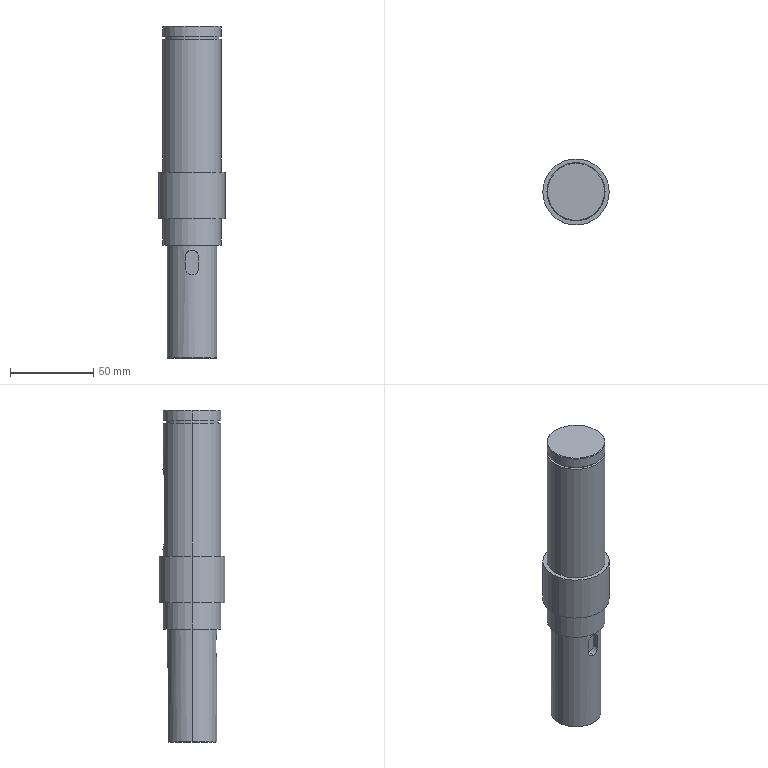Part | SolidWorks | features ICE 8, Chamfer 1, Extrusion 1 | 1 solid | 41 faces | box 40 x 40 x 200 mm | volume 179024 mm3 | cylinder 20 | plane 16 | cone 5 | commonest cylinder face diameters 35 x6 8 x5 10 x3 30 x2 32 x2 40 x2
STEP:
#1=CARTESIAN_POINT('',(-14.5,0.,0.));
#2=VERTEX_POINT('',#1);
#3=CARTESIAN_POINT('',(-4.,13.937,0.));
#4=VERTEX_POINT('',#3);
#5=CARTESIAN_POINT('',(0.,0.,0.));
#6=DIRECTION('',(0.,0.,-1.));
#7=DIRECTION('',(1.,0.,0.));
#8=AXIS2_PLACEMENT_3D('',#5,#6,#7);
#9=CIRCLE('',#8,14.5);
#10=EDGE_CURVE('',#2,#4,#9,.T.);
#11=ORIENTED_EDGE('',*,*,#10,.F.);
#12=CARTESIAN_POINT('',(-15.,0.,0.2887));
#13=VERTEX_POINT('',#12);
#14=CARTESIAN_POINT('',(-15.,0.,0.2887));
#15=DIRECTION('',(-0.866,0.,0.5));
#16=VECTOR('',#15,1000.);
#17=LINE('',#14,#16);
#18=EDGE_CURVE('',#2,#13,#17,.T.);
#19=ORIENTED_EDGE('',*,*,#18,.T.);
#20=CARTESIAN_POINT('',(-4.,14.457,0.2887));
#21=VERTEX_POINT('',#20);
#22=CARTESIAN_POINT('',(0.,0.,0.2887));
#23=DIRECTION('',(0.,0.,1.));
#24=DIRECTION('',(1.,0.,0.));
#25=AXIS2_PLACEMENT_3D('',#22,#23,#24);
#26=CIRCLE('',#25,15.);
#27=EDGE_CURVE('',#21,#13,#26,.T.);
#28=ORIENTED_EDGE('',*,*,#27,.F.);
#29=CARTESIAN_POINT('',(-4.,13.937,0.));
#30=CARTESIAN_POINT('',(-4.,14.111,0.09612));
#31=CARTESIAN_POINT('',(-4.,14.284,0.1924));
#32=CARTESIAN_POINT('',(-4.,14.457,0.2887));
#33=B_SPLINE_CURVE_WITH_KNOTS('',3,(#29,#30,#31,#32),.UNSPECIFIED.,.F.,.F.,(4,4),(0.,0.0005943),.UNSPECIFIED.);
#34=EDGE_CURVE('',#4,#21,#33,.T.);
#35=ORIENTED_EDGE('',*,*,#34,.F.);
#36=EDGE_LOOP('',(#11,#19,#28,#35));
#37=FACE_OUTER_BOUND('',#36,.T.);
#38=CARTESIAN_POINT('',(0.,0.,0.2887));
#39=DIRECTION('',(0.,0.,1.));
#40=DIRECTION('',(1.,0.,0.));
#41=AXIS2_PLACEMENT_3D('',#38,#39,#40);
#42=CONICAL_SURFACE('',#41,15.,1.047);
#43=ADVANCED_FACE('',(#37),#42,.T.);
#44=ORIENTED_EDGE('',*,*,#18,.F.);
#45=CARTESIAN_POINT('',(14.5,0.,0.));
#46=VERTEX_POINT('',#45);
#47=CARTESIAN_POINT('',(0.,0.,0.));
#48=DIRECTION('',(0.,0.,-1.));
#49=DIRECTION('',(1.,0.,0.));
#50=AXIS2_PLACEMENT_3D('',#47,#48,#49);
#51=CIRCLE('',#50,14.5);
#52=EDGE_CURVE('',#46,#2,#51,.T.);
#53=ORIENTED_EDGE('',*,*,#52,.F.);
#54=CARTESIAN_POINT('',(15.,0.,0.2887));
#55=VERTEX_POINT('',#54);
#56=CARTESIAN_POINT('',(15.,0.,0.2887));
#57=DIRECTION('',(0.866,0.,0.5));
#58=VECTOR('',#57,1000.);
#59=LINE('',#56,#58);
#60=EDGE_CURVE('',#46,#55,#59,.T.);
#61=ORIENTED_EDGE('',*,*,#60,.T.);
#62=CARTESIAN_POINT('',(0.,0.,0.2887));
#63=DIRECTION('',(0.,0.,1.));
#64=DIRECTION('',(1.,0.,0.));
#65=AXIS2_PLACEMENT_3D('',#62,#63,#64);
#66=CIRCLE('',#65,15.);
#67=EDGE_CURVE('',#13,#55,#66,.T.);
#68=ORIENTED_EDGE('',*,*,#67,.F.);
#69=EDGE_LOOP('',(#44,#53,#61,#68));
#70=FACE_OUTER_BOUND('',#69,.T.);
#71=CARTESIAN_POINT('',(0.,0.,0.2887));
#72=DIRECTION('',(0.,0.,1.));
#73=DIRECTION('',(1.,0.,0.));
#74=AXIS2_PLACEMENT_3D('',#71,#72,#73);
#75=CONICAL_SURFACE('',#74,15.,1.047);
#76=ADVANCED_FACE('',(#70),#75,.T.);
#77=CARTESIAN_POINT('',(17.211,0.,200.));
#78=VERTEX_POINT('',#77);
#79=CARTESIAN_POINT('',(-17.211,0.,200.));
#80=VERTEX_POINT('',#79);
#81=CARTESIAN_POINT('',(0.,0.,200.));
#82=DIRECTION('',(0.,0.,1.));
#83=DIRECTION('',(1.,0.,0.));
#84=AXIS2_PLACEMENT_3D('',#81,#82,#83);
#85=CIRCLE('',#84,17.211);
#86=EDGE_CURVE('',#78,#80,#85,.T.);
#87=ORIENTED_EDGE('',*,*,#86,.F.);
#88=CARTESIAN_POINT('',(17.5,0.,199.5));
#89=VERTEX_POINT('',#88);
#90=CARTESIAN_POINT('',(17.211,0.,200.));
#91=DIRECTION('',(0.5,0.,-0.866));
#92=VECTOR('',#91,1000.);
#93=LINE('',#90,#92);
#94=EDGE_CURVE('',#78,#89,#93,.T.);
#95=ORIENTED_EDGE('',*,*,#94,.T.);
#96=CARTESIAN_POINT('',(-17.5,0.,199.5));
#97=VERTEX_POINT('',#96);
#98=CARTESIAN_POINT('',(0.,0.,199.5));
#99=DIRECTION('',(0.,0.,-1.));
#100=DIRECTION('',(1.,0.,0.));
#101=AXIS2_PLACEMENT_3D('',#98,#99,#100);
#102=CIRCLE('',#101,17.5);
#103=EDGE_CURVE('',#97,#89,#102,.T.);
#104=ORIENTED_EDGE('',*,*,#103,.F.);
#105=CARTESIAN_POINT('',(-17.211,0.,200.));
#106=DIRECTION('',(-0.5,0.,-0.866));
#107=VECTOR('',#106,1000.);
#108=LINE('',#105,#107);
#109=EDGE_CURVE('',#80,#97,#108,.T.);
#110=ORIENTED_EDGE('',*,*,#109,.F.);
#111=EDGE_LOOP('',(#87,#95,#104,#110));
#112=FACE_OUTER_BOUND('',#111,.T.);
#113=CARTESIAN_POINT('',(0.,0.,200.));
#114=DIRECTION('',(0.,0.,-1.));
#115=DIRECTION('',(-1.,0.,0.));
#116=AXIS2_PLACEMENT_3D('',#113,#114,#115);
#117=CONICAL_SURFACE('',#116,17.211,0.5236);
#118=ADVANCED_FACE('',(#112),#117,.T.);
#119=CARTESIAN_POINT('',(4.,-11.,54.));
#120=VERTEX_POINT('',#119);
#121=CARTESIAN_POINT('',(0.,-11.,50.));
#122=VERTEX_POINT('',#121);
#123=CARTESIAN_POINT('',(0.,-11.,54.));
#124=DIRECTION('',(0.,1.,0.));
#125=DIRECTION('',(0.,0.,1.));
#126=AXIS2_PLACEMENT_3D('',#123,#124,#125);
#127=CIRCLE('',#126,4.);
#128=EDGE_CURVE('',#120,#122,#127,.T.);
#129=ORIENTED_EDGE('',*,*,#128,.T.);
#130=CARTESIAN_POINT('',(0.,-15.,50.));
#131=VERTEX_POINT('',#130);
#132=CARTESIAN_POINT('',(0.,-11.,50.));
#133=DIRECTION('',(0.,-1.,0.));
#134=VECTOR('',#133,1000.);
#135=LINE('',#132,#134);
#136=EDGE_CURVE('',#122,#131,#135,.T.);
#137=ORIENTED_EDGE('',*,*,#136,.T.);
#138=CARTESIAN_POINT('',(4.,-14.457,54.));
#139=VERTEX_POINT('',#138);
#140=CARTESIAN_POINT('',(0.,-15.,50.));
#141=CARTESIAN_POINT('',(0.262,-15.,50.));
#142=CARTESIAN_POINT('',(0.5282,-14.993,50.026));
#143=CARTESIAN_POINT('',(1.042,-14.966,50.129));
#144=CARTESIAN_POINT('',(1.292,-14.946,50.205));
#145=CARTESIAN_POINT('',(2.02,-14.871,50.508));
#146=CARTESIAN_POINT('',(2.459,-14.802,50.802));
#147=CARTESIAN_POINT('',(3.014,-14.695,51.357));
#148=CARTESIAN_POINT('',(3.178,-14.66,51.557));
#149=CARTESIAN_POINT('',(3.467,-14.594,51.989));
#150=CARTESIAN_POINT('',(3.593,-14.564,52.223));
#151=CARTESIAN_POINT('',(3.794,-14.513,52.705));
#152=CARTESIAN_POINT('',(3.87,-14.492,52.954));
#153=CARTESIAN_POINT('',(3.973,-14.464,53.469));
#154=CARTESIAN_POINT('',(4.,-14.457,53.735));
#155=CARTESIAN_POINT('',(4.,-14.457,54.));
#156=B_SPLINE_CURVE_WITH_KNOTS('',3,(#140,#141,#142,#143,#144,#145,#146,#147,#148,#149,#150,#151,#152,#153,#154,#155),.UNSPECIFIED.,.F.,.F.,(4,2,2,2,2,2,2,4),(0.006283,0.007068,0.007852,0.009421,0.01021,0.01099,0.01177,0.01256),.UNSPECIFIED.);
#157=EDGE_CURVE('',#131,#139,#156,.T.);
#158=ORIENTED_EDGE('',*,*,#157,.T.);
#159=CARTESIAN_POINT('',(4.,-11.,54.));
#160=DIRECTION('',(0.,-1.,0.));
#161=VECTOR('',#160,1000.);
#162=LINE('',#159,#161);
#163=EDGE_CURVE('',#120,#139,#162,.T.);
#164=ORIENTED_EDGE('',*,*,#163,.F.);
#165=EDGE_LOOP('',(#129,#137,#158,#164));
#166=FACE_OUTER_BOUND('',#165,.T.);
#167=CARTESIAN_POINT('',(0.,-11.,54.));
#168=DIRECTION('',(0.,-1.,0.));
#169=DIRECTION('',(0.,0.,-1.));
#170=AXIS2_PLACEMENT_3D('',#167,#168,#169);
#171=CYLINDRICAL_SURFACE('',#170,4.);
#172=ADVANCED_FACE('',(#166),#171,.F.);
#173=CARTESIAN_POINT('',(0.,11.,48.));
#174=VERTEX_POINT('',#173);
#175=CARTESIAN_POINT('',(4.,11.,44.));
#176=VERTEX_POINT('',#175);
#177=CARTESIAN_POINT('',(0.,11.,44.));
#178=DIRECTION('',(0.,1.,0.));
#179=DIRECTION('',(0.,0.,1.));
#180=AXIS2_PLACEMENT_3D('',#177,#178,#179);
#181=CIRCLE('',#180,4.);
#182=EDGE_CURVE('',#174,#176,#181,.T.);
#183=ORIENTED_EDGE('',*,*,#182,.F.);
#184=CARTESIAN_POINT('',(0.,15.,48.));
#185=VERTEX_POINT('',#184);
#186=CARTESIAN_POINT('',(0.,11.,48.));
#187=DIRECTION('',(0.,1.,0.));
#188=VECTOR('',#187,1000.);
#189=LINE('',#186,#188);
#190=EDGE_CURVE('',#174,#185,#189,.T.);
#191=ORIENTED_EDGE('',*,*,#190,.T.);
#192=CARTESIAN_POINT('',(4.,14.457,44.));
#193=VERTEX_POINT('',#192);
#194=CARTESIAN_POINT('',(4.,14.457,44.));
#195=CARTESIAN_POINT('',(4.,14.457,44.266));
#196=CARTESIAN_POINT('',(3.974,14.464,44.527));
#197=CARTESIAN_POINT('',(3.871,14.492,45.04));
#198=CARTESIAN_POINT('',(3.794,14.513,45.294));
#199=CARTESIAN_POINT('',(3.593,14.564,45.778));
#200=CARTESIAN_POINT('',(3.47,14.594,46.008));
#201=CARTESIAN_POINT('',(3.179,14.66,46.442));
#202=CARTESIAN_POINT('',(3.011,14.696,46.646));
#203=CARTESIAN_POINT('',(2.644,14.766,47.013));
#204=CARTESIAN_POINT('',(2.443,14.801,47.178));
#205=CARTESIAN_POINT('',(2.006,14.867,47.471));
#206=CARTESIAN_POINT('',(1.775,14.897,47.594));
#207=CARTESIAN_POINT('',(1.293,14.946,47.794));
#208=CARTESIAN_POINT('',(1.04,14.966,47.871));
#209=CARTESIAN_POINT('',(0.5228,14.993,47.974));
#210=CARTESIAN_POINT('',(0.2623,15.,48.));
#211=CARTESIAN_POINT('',(0.,15.,48.));
#212=B_SPLINE_CURVE_WITH_KNOTS('',3,(#194,#195,#196,#197,#198,#199,#200,#201,#202,#203,#204,#205,#206,#207,#208,#209,#210,#211),.UNSPECIFIED.,.F.,.F.,(4,2,2,2,2,2,2,2,4),(0.,0.0007854,0.001571,0.002356,0.003142,0.003927,0.004712,0.005498,0.006283),.UNSPECIFIED.);
#213=EDGE_CURVE('',#193,#185,#212,.T.);
#214=ORIENTED_EDGE('',*,*,#213,.F.);
#215=CARTESIAN_POINT('',(4.,11.,44.));
#216=DIRECTION('',(0.,1.,0.));
#217=VECTOR('',#216,1000.);
#218=LINE('',#215,#217);
#219=EDGE_CURVE('',#176,#193,#218,.T.);
#220=ORIENTED_EDGE('',*,*,#219,.F.);
#221=EDGE_LOOP('',(#183,#191,#214,#220));
#222=FACE_OUTER_BOUND('',#221,.T.);
#223=CARTESIAN_POINT('',(0.,11.,44.));
#224=DIRECTION('',(0.,1.,0.));
#225=DIRECTION('',(0.,0.,1.));
#226=AXIS2_PLACEMENT_3D('',#223,#224,#225);
#227=CYLINDRICAL_SURFACE('',#226,4.);
#228=ADVANCED_FACE('',(#222),#227,.F.);
#229=CARTESIAN_POINT('',(0.,12.5,164.));
#230=VERTEX_POINT('',#229);
#231=CARTESIAN_POINT('',(5.,12.5,159.));
#232=VERTEX_POINT('',#231);
#233=CARTESIAN_POINT('',(0.,12.5,159.));
#234=DIRECTION('',(0.,1.,0.));
#235=DIRECTION('',(0.,0.,1.));
#236=AXIS2_PLACEMENT_3D('',#233,#234,#235);
#237=CIRCLE('',#236,5.);
#238=EDGE_CURVE('',#230,#232,#237,.T.);
#239=ORIENTED_EDGE('',*,*,#238,.F.);
#240=CARTESIAN_POINT('',(0.,17.5,164.));
#241=VERTEX_POINT('',#240);
#242=CARTESIAN_POINT('',(0.,12.5,164.));
#243=DIRECTION('',(0.,1.,0.));
#244=VECTOR('',#243,1000.);
#245=LINE('',#242,#244);
#246=EDGE_CURVE('',#230,#241,#245,.T.);
#247=ORIENTED_EDGE('',*,*,#246,.T.);
#248=CARTESIAN_POINT('',(5.,16.771,159.));
#249=VERTEX_POINT('',#248);
#250=CARTESIAN_POINT('',(5.,16.771,159.));
#251=CARTESIAN_POINT('',(5.,16.771,159.332));
#252=CARTESIAN_POINT('',(4.967,16.78,159.659));
#253=CARTESIAN_POINT('',(4.839,16.818,160.3));
#254=CARTESIAN_POINT('',(4.742,16.846,160.619));
#255=CARTESIAN_POINT('',(4.49,16.915,161.224));
#256=CARTESIAN_POINT('',(4.337,16.955,161.51));
#257=CARTESIAN_POINT('',(3.974,17.044,162.052));
#258=CARTESIAN_POINT('',(3.764,17.092,162.308));
#259=CARTESIAN_POINT('',(3.305,17.187,162.766));
#260=CARTESIAN_POINT('',(3.054,17.234,162.973));
#261=CARTESIAN_POINT('',(2.507,17.322,163.338));
#262=CARTESIAN_POINT('',(2.219,17.361,163.492));
#263=CARTESIAN_POINT('',(1.768,17.411,163.68));
#264=CARTESIAN_POINT('',(1.614,17.426,163.735));
#265=CARTESIAN_POINT('',(1.3,17.452,163.831));
#266=CARTESIAN_POINT('',(1.139,17.464,163.871));
#267=CARTESIAN_POINT('',(0.6539,17.491,163.968));
#268=CARTESIAN_POINT('',(0.3282,17.5,164.));
#269=CARTESIAN_POINT('',(0.,17.5,164.));
#270=B_SPLINE_CURVE_WITH_KNOTS('',3,(#250,#251,#252,#253,#254,#255,#256,#257,#258,#259,#260,#261,#262,#263,#264,#265,#266,#267,#268,#269),.UNSPECIFIED.,.F.,.F.,(4,2,2,2,2,2,2,2,2,4),(0.,0.0009824,0.001965,0.002947,0.00393,0.004912,0.005894,0.006386,0.006877,0.007859),.UNSPECIFIED.);
#271=EDGE_CURVE('',#249,#241,#270,.T.);
#272=ORIENTED_EDGE('',*,*,#271,.F.);
#273=CARTESIAN_POINT('',(5.,12.5,159.));
#274=DIRECTION('',(0.,1.,0.));
#275=VECTOR('',#274,1000.);
#276=LINE('',#273,#275);
#277=EDGE_CURVE('',#232,#249,#276,.T.);
#278=ORIENTED_EDGE('',*,*,#277,.F.);
#279=EDGE_LOOP('',(#239,#247,#272,#278));
#280=FACE_OUTER_BOUND('',#279,.T.);
#281=CARTESIAN_POINT('',(0.,12.5,159.));
#282=DIRECTION('',(0.,1.,0.));
#283=DIRECTION('',(0.,0.,1.));
#284=AXIS2_PLACEMENT_3D('',#281,#282,#283);
#285=CYLINDRICAL_SURFACE('',#284,5.);
#286=ADVANCED_FACE('',(#280),#285,.F.);
#287=ORIENTED_EDGE('',*,*,#103,.T.);
#288=CARTESIAN_POINT('',(17.5,0.,193.5));
#289=VERTEX_POINT('',#288);
#290=CARTESIAN_POINT('',(17.5,0.,200.));
#291=DIRECTION('',(0.,0.,-1.));
#292=VECTOR('',#291,1000.);
#293=LINE('',#290,#292);
#294=EDGE_CURVE('',#89,#289,#293,.T.);
#295=ORIENTED_EDGE('',*,*,#294,.T.);
#296=CARTESIAN_POINT('',(-17.5,0.,193.5));
#297=VERTEX_POINT('',#296);
#298=CARTESIAN_POINT('',(0.,0.,193.5));
#299=DIRECTION('',(0.,0.,1.));
#300=DIRECTION('',(1.,0.,0.));
#301=AXIS2_PLACEMENT_3D('',#298,#299,#300);
#302=CIRCLE('',#301,17.5);
#303=EDGE_CURVE('',#289,#297,#302,.T.);
#304=ORIENTED_EDGE('',*,*,#303,.T.);
#305=CARTESIAN_POINT('',(-17.5,0.,200.));
#306=DIRECTION('',(0.,0.,-1.));
#307=VECTOR('',#306,1000.);
#308=LINE('',#305,#307);
#309=EDGE_CURVE('',#97,#297,#308,.T.);
#310=ORIENTED_EDGE('',*,*,#309,.F.);
#311=EDGE_LOOP('',(#287,#295,#304,#310));
#312=FACE_OUTER_BOUND('',#311,.T.);
#313=CARTESIAN_POINT('',(0.,0.,200.));
#314=DIRECTION('',(0.,0.,-1.));
#315=DIRECTION('',(-1.,0.,0.));
#316=AXIS2_PLACEMENT_3D('',#313,#314,#315);
#317=CYLINDRICAL_SURFACE('',#316,17.5);
#318=ADVANCED_FACE('',(#312),#317,.T.);
#319=CARTESIAN_POINT('',(16.,0.,193.5));
#320=VERTEX_POINT('',#319);
#321=CARTESIAN_POINT('',(-16.,0.,193.5));
#322=VERTEX_POINT('',#321);
#323=CARTESIAN_POINT('',(0.,0.,193.5));
#324=DIRECTION('',(0.,0.,1.));
#325=DIRECTION('',(1.,0.,0.));
#326=AXIS2_PLACEMENT_3D('',#323,#324,#325);
#327=CIRCLE('',#326,16.);
#328=EDGE_CURVE('',#320,#322,#327,.T.);
#329=ORIENTED_EDGE('',*,*,#328,.F.);
#330=CARTESIAN_POINT('',(16.,0.,192.));
#331=VERTEX_POINT('',#330);
#332=CARTESIAN_POINT('',(16.,0.,193.5));
#333=DIRECTION('',(0.,0.,-1.));
#334=VECTOR('',#333,1000.);
#335=LINE('',#332,#334);
#336=EDGE_CURVE('',#320,#331,#335,.T.);
#337=ORIENTED_EDGE('',*,*,#336,.T.);
#338=CARTESIAN_POINT('',(-16.,0.,192.));
#339=VERTEX_POINT('',#338);
#340=CARTESIAN_POINT('',(0.,0.,192.));
#341=DIRECTION('',(0.,0.,1.));
#342=DIRECTION('',(1.,0.,0.));
#343=AXIS2_PLACEMENT_3D('',#340,#341,#342);
#344=CIRCLE('',#343,16.);
#345=EDGE_CURVE('',#331,#339,#344,.T.);
#346=ORIENTED_EDGE('',*,*,#345,.T.);
#347=CARTESIAN_POINT('',(-16.,0.,193.5));
#348=DIRECTION('',(0.,0.,-1.));
#349=VECTOR('',#348,1000.);
#350=LINE('',#347,#349);
#351=EDGE_CURVE('',#322,#339,#350,.T.);
#352=ORIENTED_EDGE('',*,*,#351,.F.);
#353=EDGE_LOOP('',(#329,#337,#346,#352));
#354=FACE_OUTER_BOUND('',#353,.T.);
#355=CARTESIAN_POINT('',(0.,0.,193.5));
#356=DIRECTION('',(0.,0.,-1.));
#357=DIRECTION('',(-1.,0.,0.));
#358=AXIS2_PLACEMENT_3D('',#355,#356,#357);
#359=CYLINDRICAL_SURFACE('',#358,16.);
#360=ADVANCED_FACE('',(#354),#359,.T.);
#361=CARTESIAN_POINT('',(-5.,16.771,159.));
#362=VERTEX_POINT('',#361);
#363=CARTESIAN_POINT('',(-5.,16.771,121.));
#364=VERTEX_POINT('',#363);
#365=CARTESIAN_POINT('',(-5.,16.771,192.));
#366=DIRECTION('',(0.,0.,-1.));
#367=VECTOR('',#366,1000.);
#368=LINE('',#365,#367);
#369=EDGE_CURVE('',#362,#364,#368,.T.);
#370=ORIENTED_EDGE('',*,*,#369,.T.);
#371=CARTESIAN_POINT('',(5.,16.771,121.));
#372=VERTEX_POINT('',#371);
#373=CARTESIAN_POINT('',(-5.,16.771,121.));
#374=CARTESIAN_POINT('',(-5.,16.771,120.668));
#375=CARTESIAN_POINT('',(-4.967,16.78,120.342));
#376=CARTESIAN_POINT('',(-4.839,16.818,119.7));
#377=CARTESIAN_POINT('',(-4.742,16.846,119.382));
#378=CARTESIAN_POINT('',(-4.491,16.914,118.778));
#379=CARTESIAN_POINT('',(-4.337,16.955,118.491));
#380=CARTESIAN_POINT('',(-3.975,17.044,117.949));
#381=CARTESIAN_POINT('',(-3.765,17.092,117.694));
#382=CARTESIAN_POINT('',(-3.306,17.186,117.235));
#383=CARTESIAN_POINT('',(-3.056,17.233,117.029));
#384=CARTESIAN_POINT('',(-2.51,17.321,116.663));
#385=CARTESIAN_POINT('',(-2.222,17.361,116.509));
#386=CARTESIAN_POINT('',(-1.771,17.411,116.321));
#387=CARTESIAN_POINT('',(-1.618,17.426,116.266));
#388=CARTESIAN_POINT('',(-1.304,17.452,116.17));
#389=CARTESIAN_POINT('',(-1.143,17.463,116.13));
#390=CARTESIAN_POINT('',(-0.6583,17.491,116.033));
#391=CARTESIAN_POINT('',(-0.3328,17.5,116.));
#392=CARTESIAN_POINT('',(0.3232,17.5,116.));
#393=CARTESIAN_POINT('',(0.6564,17.491,116.032));
#394=CARTESIAN_POINT('',(1.299,17.455,116.161));
#395=CARTESIAN_POINT('',(1.612,17.428,116.255));
#396=CARTESIAN_POINT('',(2.219,17.361,116.507));
#397=CARTESIAN_POINT('',(2.509,17.321,116.663));
#398=CARTESIAN_POINT('',(3.049,17.235,117.024));
#399=CARTESIAN_POINT('',(3.303,17.187,117.232));
#400=CARTESIAN_POINT('',(3.765,17.092,117.694));
#401=CARTESIAN_POINT('',(3.971,17.045,117.945));
#402=CARTESIAN_POINT('',(4.333,16.956,118.484));
#403=CARTESIAN_POINT('',(4.49,16.915,118.777));
#404=CARTESIAN_POINT('',(4.741,16.846,119.379));
#405=CARTESIAN_POINT('',(4.837,16.818,119.691));
#406=CARTESIAN_POINT('',(4.967,16.781,120.336));
#407=CARTESIAN_POINT('',(5.,16.771,120.668));
#408=CARTESIAN_POINT('',(5.,16.771,121.));
#409=B_SPLINE_CURVE_WITH_KNOTS('',3,(#373,#374,#375,#376,#377,#378,#379,#380,#381,#382,#383,#384,#385,#386,#387,#388,#389,#390,#391,#392,#393,#394,#395,#396,#397,#398,#399,#400,#401,#402,#403,#404,#405,#406,#407,#408),.UNSPECIFIED.,.F.,.F.,(4,2,2,2,2,2,2,2,2,2,2,2,2,2,2,2,2,4),(0.,0.0009818,0.001964,0.002945,0.003927,0.004909,0.005891,0.006382,0.006873,0.007855,0.008836,0.009818,0.0108,0.01178,0.01276,0.01375,0.01473,0.01571),.UNSPECIFIED.);
#410=EDGE_CURVE('',#364,#372,#409,.T.);
#411=ORIENTED_EDGE('',*,*,#410,.T.);
#412=CARTESIAN_POINT('',(5.,16.771,192.));
#413=DIRECTION('',(0.,0.,1.));
#414=VECTOR('',#413,1000.);
#415=LINE('',#412,#414);
#416=EDGE_CURVE('',#372,#249,#415,.T.);
#417=ORIENTED_EDGE('',*,*,#416,.T.);
#418=ORIENTED_EDGE('',*,*,#271,.T.);
#419=CARTESIAN_POINT('',(0.,17.5,164.));
#420=CARTESIAN_POINT('',(-0.3278,17.5,164.));
#421=CARTESIAN_POINT('',(-0.6608,17.49,163.967));
#422=CARTESIAN_POINT('',(-1.303,17.454,163.838));
#423=CARTESIAN_POINT('',(-1.615,17.428,163.743));
#424=CARTESIAN_POINT('',(-2.222,17.361,163.491));
#425=CARTESIAN_POINT('',(-2.512,17.321,163.335));
#426=CARTESIAN_POINT('',(-3.051,17.234,162.974));
#427=CARTESIAN_POINT('',(-3.305,17.187,162.766));
#428=CARTESIAN_POINT('',(-3.767,17.091,162.304));
#429=CARTESIAN_POINT('',(-3.972,17.044,162.054));
#430=CARTESIAN_POINT('',(-4.334,16.956,161.514));
#431=CARTESIAN_POINT('',(-4.491,16.914,161.222));
#432=CARTESIAN_POINT('',(-4.742,16.846,160.62));
#433=CARTESIAN_POINT('',(-4.837,16.818,160.308));
#434=CARTESIAN_POINT('',(-4.967,16.781,159.664));
#435=CARTESIAN_POINT('',(-5.,16.771,159.332));
#436=CARTESIAN_POINT('',(-5.,16.771,159.));
#437=B_SPLINE_CURVE_WITH_KNOTS('',3,(#419,#420,#421,#422,#423,#424,#425,#426,#427,#428,#429,#430,#431,#432,#433,#434,#435,#436),.UNSPECIFIED.,.F.,.F.,(4,2,2,2,2,2,2,2,4),(0.007859,0.008841,0.009822,0.0108,0.01178,0.01277,0.01375,0.01473,0.01571),.UNSPECIFIED.);
#438=EDGE_CURVE('',#241,#362,#437,.T.);
#439=ORIENTED_EDGE('',*,*,#438,.T.);
#440=EDGE_LOOP('',(#370,#411,#417,#418,#439));
#441=FACE_BOUND('',#440,.T.);
#442=CARTESIAN_POINT('',(17.5,0.,192.));
#443=VERTEX_POINT('',#442);
#444=CARTESIAN_POINT('',(-17.5,0.,192.));
#445=VERTEX_POINT('',#444);
#446=CARTESIAN_POINT('',(0.,0.,192.));
#447=DIRECTION('',(0.,0.,1.));
#448=DIRECTION('',(1.,0.,0.));
#449=AXIS2_PLACEMENT_3D('',#446,#447,#448);
#450=CIRCLE('',#449,17.5);
#451=EDGE_CURVE('',#443,#445,#450,.T.);
#452=ORIENTED_EDGE('',*,*,#451,.F.);
#453=CARTESIAN_POINT('',(17.5,0.,112.));
#454=VERTEX_POINT('',#453);
#455=CARTESIAN_POINT('',(17.5,0.,192.));
#456=DIRECTION('',(0.,0.,-1.));
#457=VECTOR('',#456,1000.);
#458=LINE('',#455,#457);
#459=EDGE_CURVE('',#443,#454,#458,.T.);
#460=ORIENTED_EDGE('',*,*,#459,.T.);
#461=CARTESIAN_POINT('',(-17.5,0.,112.));
#462=VERTEX_POINT('',#461);
#463=CARTESIAN_POINT('',(0.,0.,112.));
#464=DIRECTION('',(0.,0.,1.));
#465=DIRECTION('',(1.,0.,0.));
#466=AXIS2_PLACEMENT_3D('',#463,#464,#465);
#467=CIRCLE('',#466,17.5);
#468=EDGE_CURVE('',#454,#462,#467,.T.);
#469=ORIENTED_EDGE('',*,*,#468,.T.);
#470=CARTESIAN_POINT('',(-17.5,0.,192.));
#471=DIRECTION('',(0.,0.,-1.));
#472=VECTOR('',#471,1000.);
#473=LINE('',#470,#472);
#474=EDGE_CURVE('',#445,#462,#473,.T.);
#475=ORIENTED_EDGE('',*,*,#474,.F.);
#476=EDGE_LOOP('',(#452,#460,#469,#475));
#477=FACE_OUTER_BOUND('',#476,.T.);
#478=CARTESIAN_POINT('',(0.,0.,192.));
#479=DIRECTION('',(0.,0.,-1.));
#480=DIRECTION('',(-1.,0.,0.));
#481=AXIS2_PLACEMENT_3D('',#478,#479,#480);
#482=CYLINDRICAL_SURFACE('',#481,17.5);
#483=ADVANCED_FACE('',(#441,#477),#482,.T.);
#484=CARTESIAN_POINT('',(20.,0.,112.));
#485=VERTEX_POINT('',#484);
#486=CARTESIAN_POINT('',(-20.,0.,112.));
#487=VERTEX_POINT('',#486);
#488=CARTESIAN_POINT('',(0.,0.,112.));
#489=DIRECTION('',(0.,0.,1.));
#490=DIRECTION('',(1.,0.,0.));
#491=AXIS2_PLACEMENT_3D('',#488,#489,#490);
#492=CIRCLE('',#491,20.);
#493=EDGE_CURVE('',#485,#487,#492,.T.);
#494=ORIENTED_EDGE('',*,*,#493,.F.);
#495=CARTESIAN_POINT('',(20.,0.,84.));
#496=VERTEX_POINT('',#495);
#497=CARTESIAN_POINT('',(20.,0.,112.));
#498=DIRECTION('',(0.,0.,-1.));
#499=VECTOR('',#498,1000.);
#500=LINE('',#497,#499);
#501=EDGE_CURVE('',#485,#496,#500,.T.);
#502=ORIENTED_EDGE('',*,*,#501,.T.);
#503=CARTESIAN_POINT('',(-20.,0.,84.));
#504=VERTEX_POINT('',#503);
#505=CARTESIAN_POINT('',(0.,0.,84.));
#506=DIRECTION('',(0.,0.,1.));
#507=DIRECTION('',(1.,0.,0.));
#508=AXIS2_PLACEMENT_3D('',#505,#506,#507);
#509=CIRCLE('',#508,20.);
#510=EDGE_CURVE('',#496,#504,#509,.T.);
#511=ORIENTED_EDGE('',*,*,#510,.T.);
#512=CARTESIAN_POINT('',(-20.,0.,112.));
#513=DIRECTION('',(0.,0.,-1.));
#514=VECTOR('',#513,1000.);
#515=LINE('',#512,#514);
#516=EDGE_CURVE('',#487,#504,#515,.T.);
#517=ORIENTED_EDGE('',*,*,#516,.F.);
#518=EDGE_LOOP('',(#494,#502,#511,#517));
#519=FACE_OUTER_BOUND('',#518,.T.);
#520=CARTESIAN_POINT('',(0.,0.,112.));
#521=DIRECTION('',(0.,0.,-1.));
#522=DIRECTION('',(-1.,0.,0.));
#523=AXIS2_PLACEMENT_3D('',#520,#521,#522);
#524=CYLINDRICAL_SURFACE('',#523,20.);
#525=ADVANCED_FACE('',(#519),#524,.T.);
#526=CARTESIAN_POINT('',(17.5,0.,84.));
#527=VERTEX_POINT('',#526);
#528=CARTESIAN_POINT('',(-17.5,0.,84.));
#529=VERTEX_POINT('',#528);
#530=CARTESIAN_POINT('',(0.,0.,84.));
#531=DIRECTION('',(0.,0.,1.));
#532=DIRECTION('',(1.,0.,0.));
#533=AXIS2_PLACEMENT_3D('',#530,#531,#532);
#534=CIRCLE('',#533,17.5);
#535=EDGE_CURVE('',#527,#529,#534,.T.);
#536=ORIENTED_EDGE('',*,*,#535,.F.);
#537=CARTESIAN_POINT('',(17.5,0.,68.));
#538=VERTEX_POINT('',#537);
#539=CARTESIAN_POINT('',(17.5,0.,84.));
#540=DIRECTION('',(0.,0.,-1.));
#541=VECTOR('',#540,1000.);
#542=LINE('',#539,#541);
#543=EDGE_CURVE('',#527,#538,#542,.T.);
#544=ORIENTED_EDGE('',*,*,#543,.T.);
#545=CARTESIAN_POINT('',(-17.5,0.,68.));
#546=VERTEX_POINT('',#545);
#547=CARTESIAN_POINT('',(0.,0.,68.));
#548=DIRECTION('',(0.,0.,1.));
#549=DIRECTION('',(1.,0.,0.));
#550=AXIS2_PLACEMENT_3D('',#547,#548,#549);
#551=CIRCLE('',#550,17.5);
#552=EDGE_CURVE('',#538,#546,#551,.T.);
#553=ORIENTED_EDGE('',*,*,#552,.T.);
#554=CARTESIAN_POINT('',(-17.5,0.,84.));
#555=DIRECTION('',(0.,0.,-1.));
#556=VECTOR('',#555,1000.);
#557=LINE('',#554,#556);
#558=EDGE_CURVE('',#529,#546,#557,.T.);
#559=ORIENTED_EDGE('',*,*,#558,.F.);
#560=EDGE_LOOP('',(#536,#544,#553,#559));
#561=FACE_OUTER_BOUND('',#560,.T.);
#562=CARTESIAN_POINT('',(0.,0.,84.));
#563=DIRECTION('',(0.,0.,-1.));
#564=DIRECTION('',(-1.,0.,0.));
#565=AXIS2_PLACEMENT_3D('',#562,#563,#564);
#566=CYLINDRICAL_SURFACE('',#565,17.5);
#567=ADVANCED_FACE('',(#561),#566,.T.);
#568=CARTESIAN_POINT('',(15.,0.,68.));
#569=VERTEX_POINT('',#568);
#570=CARTESIAN_POINT('',(-15.,0.,68.));
#571=VERTEX_POINT('',#570);
#572=CARTESIAN_POINT('',(0.,0.,68.));
#573=DIRECTION('',(0.,0.,1.));
#574=DIRECTION('',(1.,0.,0.));
#575=AXIS2_PLACEMENT_3D('',#572,#573,#574);
#576=CIRCLE('',#575,15.);
#577=EDGE_CURVE('',#569,#571,#576,.T.);
#578=ORIENTED_EDGE('',*,*,#577,.F.);
#579=CARTESIAN_POINT('',(15.,0.,68.));
#580=DIRECTION('',(0.,0.,-1.));
#581=VECTOR('',#580,1000.);
#582=LINE('',#579,#581);
#583=EDGE_CURVE('',#569,#55,#582,.T.);
#584=ORIENTED_EDGE('',*,*,#583,.T.);
#585=CARTESIAN_POINT('',(4.,14.457,0.2887));
#586=VERTEX_POINT('',#585);
#587=CARTESIAN_POINT('',(0.,0.,0.2887));
#588=DIRECTION('',(0.,0.,1.));
#589=DIRECTION('',(1.,0.,0.));
#590=AXIS2_PLACEMENT_3D('',#587,#588,#589);
#591=CIRCLE('',#590,15.);
#592=EDGE_CURVE('',#55,#586,#591,.T.);
#593=ORIENTED_EDGE('',*,*,#592,.T.);
#594=CARTESIAN_POINT('',(4.,14.457,68.));
#595=DIRECTION('',(0.,0.,1.));
#596=VECTOR('',#595,1000.);
#597=LINE('',#594,#596);
#598=EDGE_CURVE('',#586,#193,#597,.T.);
#599=ORIENTED_EDGE('',*,*,#598,.T.);
#600=ORIENTED_EDGE('',*,*,#213,.T.);
#601=CARTESIAN_POINT('',(-4.,14.457,44.));
#602=VERTEX_POINT('',#601);
#603=CARTESIAN_POINT('',(0.,15.,48.));
#604=CARTESIAN_POINT('',(-0.262,15.,48.));
#605=CARTESIAN_POINT('',(-0.5282,14.993,47.974));
#606=CARTESIAN_POINT('',(-1.042,14.966,47.871));
#607=CARTESIAN_POINT('',(-1.292,14.946,47.795));
#608=CARTESIAN_POINT('',(-2.02,14.871,47.492));
#609=CARTESIAN_POINT('',(-2.459,14.802,47.198));
#610=CARTESIAN_POINT('',(-3.014,14.695,46.643));
#611=CARTESIAN_POINT('',(-3.178,14.66,46.443));
#612=CARTESIAN_POINT('',(-3.467,14.594,46.011));
#613=CARTESIAN_POINT('',(-3.593,14.564,45.777));
#614=CARTESIAN_POINT('',(-3.794,14.513,45.295));
#615=CARTESIAN_POINT('',(-3.87,14.492,45.046));
#616=CARTESIAN_POINT('',(-3.973,14.464,44.531));
#617=CARTESIAN_POINT('',(-4.,14.457,44.265));
#618=CARTESIAN_POINT('',(-4.,14.457,44.));
#619=B_SPLINE_CURVE_WITH_KNOTS('',3,(#603,#604,#605,#606,#607,#608,#609,#610,#611,#612,#613,#614,#615,#616,#617,#618),.UNSPECIFIED.,.F.,.F.,(4,2,2,2,2,2,2,4),(0.006283,0.007068,0.007852,0.009421,0.01021,0.01099,0.01177,0.01256),.UNSPECIFIED.);
#620=EDGE_CURVE('',#185,#602,#619,.T.);
#621=ORIENTED_EDGE('',*,*,#620,.T.);
#622=CARTESIAN_POINT('',(-4.,14.457,68.));
#623=DIRECTION('',(0.,0.,-1.));
#624=VECTOR('',#623,1000.);
#625=LINE('',#622,#624);
#626=EDGE_CURVE('',#602,#21,#625,.T.);
#627=ORIENTED_EDGE('',*,*,#626,.T.);
#628=ORIENTED_EDGE('',*,*,#27,.T.);
#629=CARTESIAN_POINT('',(-15.,0.,68.));
#630=DIRECTION('',(0.,0.,-1.));
#631=VECTOR('',#630,1000.);
#632=LINE('',#629,#631);
#633=EDGE_CURVE('',#571,#13,#632,.T.);
#634=ORIENTED_EDGE('',*,*,#633,.F.);
#635=EDGE_LOOP('',(#578,#584,#593,#599,#600,#621,#627,#628,#634));
#636=FACE_OUTER_BOUND('',#635,.T.);
#637=CARTESIAN_POINT('',(0.,0.,68.));
#638=DIRECTION('',(0.,0.,-1.));
#639=DIRECTION('',(-1.,0.,0.));
#640=AXIS2_PLACEMENT_3D('',#637,#638,#639);
#641=CYLINDRICAL_SURFACE('',#640,15.);
#642=ADVANCED_FACE('',(#636),#641,.T.);
#643=ORIENTED_EDGE('',*,*,#583,.F.);
#644=CARTESIAN_POINT('',(0.,0.,68.));
#645=DIRECTION('',(0.,0.,1.));
#646=DIRECTION('',(1.,0.,0.));
#647=AXIS2_PLACEMENT_3D('',#644,#645,#646);
#648=CIRCLE('',#647,15.);
#649=EDGE_CURVE('',#571,#569,#648,.T.);
#650=ORIENTED_EDGE('',*,*,#649,.F.);
#651=ORIENTED_EDGE('',*,*,#633,.T.);
#652=ORIENTED_EDGE('',*,*,#67,.T.);
#653=EDGE_LOOP('',(#643,#650,#651,#652));
#654=FACE_OUTER_BOUND('',#653,.T.);
#655=CARTESIAN_POINT('',(-4.,-14.457,54.));
#656=VERTEX_POINT('',#655);
#657=CARTESIAN_POINT('',(-4.,-14.457,54.));
#658=CARTESIAN_POINT('',(-4.,-14.457,53.734));
#659=CARTESIAN_POINT('',(-3.974,-14.464,53.473));
#660=CARTESIAN_POINT('',(-3.871,-14.492,52.96));
#661=CARTESIAN_POINT('',(-3.794,-14.513,52.706));
#662=CARTESIAN_POINT('',(-3.593,-14.564,52.222));
#663=CARTESIAN_POINT('',(-3.47,-14.594,51.992));
#664=CARTESIAN_POINT('',(-3.179,-14.66,51.558));
#665=CARTESIAN_POINT('',(-3.011,-14.696,51.354));
#666=CARTESIAN_POINT('',(-2.644,-14.766,50.987));
#667=CARTESIAN_POINT('',(-2.443,-14.801,50.822));
#668=CARTESIAN_POINT('',(-2.006,-14.867,50.529));
#669=CARTESIAN_POINT('',(-1.775,-14.897,50.406));
#670=CARTESIAN_POINT('',(-1.293,-14.946,50.206));
#671=CARTESIAN_POINT('',(-1.04,-14.966,50.129));
#672=CARTESIAN_POINT('',(-0.5228,-14.993,50.026));
#673=CARTESIAN_POINT('',(-0.2623,-15.,50.));
#674=CARTESIAN_POINT('',(0.,-15.,50.));
#675=B_SPLINE_CURVE_WITH_KNOTS('',3,(#657,#658,#659,#660,#661,#662,#663,#664,#665,#666,#667,#668,#669,#670,#671,#672,#673,#674),.UNSPECIFIED.,.F.,.F.,(4,2,2,2,2,2,2,2,4),(0.,0.0007854,0.001571,0.002356,0.003142,0.003927,0.004712,0.005498,0.006283),.UNSPECIFIED.);
#676=EDGE_CURVE('',#656,#131,#675,.T.);
#677=ORIENTED_EDGE('',*,*,#676,.F.);
#678=CARTESIAN_POINT('',(-4.,-14.457,61.));
#679=VERTEX_POINT('',#678);
#680=CARTESIAN_POINT('',(-4.,-14.457,68.));
#681=DIRECTION('',(0.,0.,-1.));
#682=VECTOR('',#681,1000.);
#683=LINE('',#680,#682);
#684=EDGE_CURVE('',#679,#656,#683,.T.);
#685=ORIENTED_EDGE('',*,*,#684,.F.);
#686=CARTESIAN_POINT('',(4.,-14.457,61.));
#687=VERTEX_POINT('',#686);
#688=CARTESIAN_POINT('',(4.,-14.457,61.));
#689=CARTESIAN_POINT('',(4.,-14.457,61.266));
#690=CARTESIAN_POINT('',(3.974,-14.464,61.526));
#691=CARTESIAN_POINT('',(3.872,-14.492,62.039));
#692=CARTESIAN_POINT('',(3.794,-14.513,62.294));
#693=CARTESIAN_POINT('',(3.593,-14.564,62.777));
#694=CARTESIAN_POINT('',(3.47,-14.594,63.007));
#695=CARTESIAN_POINT('',(3.18,-14.66,63.44));
#696=CARTESIAN_POINT('',(3.012,-14.696,63.645));
#697=CARTESIAN_POINT('',(2.645,-14.766,64.012));
#698=CARTESIAN_POINT('',(2.444,-14.801,64.177));
#699=CARTESIAN_POINT('',(2.008,-14.867,64.47));
#700=CARTESIAN_POINT('',(1.777,-14.896,64.593));
#701=CARTESIAN_POINT('',(1.296,-14.946,64.793));
#702=CARTESIAN_POINT('',(1.043,-14.966,64.871));
#703=CARTESIAN_POINT('',(0.5261,-14.993,64.974));
#704=CARTESIAN_POINT('',(0.2658,-15.,65.));
#705=CARTESIAN_POINT('',(-0.2585,-15.,65.));
#706=CARTESIAN_POINT('',(-0.5249,-14.993,64.974));
#707=CARTESIAN_POINT('',(-1.039,-14.966,64.872));
#708=CARTESIAN_POINT('',(-1.289,-14.947,64.796));
#709=CARTESIAN_POINT('',(-2.017,-14.872,64.494));
#710=CARTESIAN_POINT('',(-2.457,-14.802,64.199));
#711=CARTESIAN_POINT('',(-3.012,-14.696,63.645));
#712=CARTESIAN_POINT('',(-3.177,-14.66,63.444));
#713=CARTESIAN_POINT('',(-3.467,-14.595,63.012));
#714=CARTESIAN_POINT('',(-3.593,-14.564,62.778));
#715=CARTESIAN_POINT('',(-3.793,-14.513,62.296));
#716=CARTESIAN_POINT('',(-3.87,-14.492,62.046));
#717=CARTESIAN_POINT('',(-3.973,-14.464,61.531));
#718=CARTESIAN_POINT('',(-4.,-14.457,61.266));
#719=CARTESIAN_POINT('',(-4.,-14.457,61.));
#720=B_SPLINE_CURVE_WITH_KNOTS('',3,(#688,#689,#690,#691,#692,#693,#694,#695,#696,#697,#698,#699,#700,#701,#702,#703,#704,#705,#706,#707,#708,#709,#710,#711,#712,#713,#714,#715,#716,#717,#718,#719),.UNSPECIFIED.,.F.,.F.,(4,2,2,2,2,2,2,2,2,2,2,2,2,2,2,4),(0.,0.0007849,0.00157,0.002355,0.00314,0.003925,0.00471,0.005494,0.006279,0.007064,0.007849,0.009419,0.0102,0.01099,0.01177,0.01256),.UNSPECIFIED.);
#721=EDGE_CURVE('',#687,#679,#720,.T.);
#722=ORIENTED_EDGE('',*,*,#721,.F.);
#723=CARTESIAN_POINT('',(4.,-14.457,68.));
#724=DIRECTION('',(0.,0.,1.));
#725=VECTOR('',#724,1000.);
#726=LINE('',#723,#725);
#727=EDGE_CURVE('',#139,#687,#726,.T.);
#728=ORIENTED_EDGE('',*,*,#727,.F.);
#729=ORIENTED_EDGE('',*,*,#157,.F.);
#730=EDGE_LOOP('',(#677,#685,#722,#728,#729));
#731=FACE_BOUND('',#730,.T.);
#732=CARTESIAN_POINT('',(0.,0.,68.));
#733=DIRECTION('',(0.,0.,-1.));
#734=DIRECTION('',(-1.,0.,0.));
#735=AXIS2_PLACEMENT_3D('',#732,#733,#734);
#736=CYLINDRICAL_SURFACE('',#735,15.);
#737=ADVANCED_FACE('',(#654,#731),#736,.T.);
#738=CARTESIAN_POINT('',(4.,11.,0.));
#739=VERTEX_POINT('',#738);
#740=CARTESIAN_POINT('',(4.,13.937,0.));
#741=VERTEX_POINT('',#740);
#742=CARTESIAN_POINT('',(4.,11.,0.));
#743=DIRECTION('',(0.,1.,0.));
#744=VECTOR('',#743,1000.);
#745=LINE('',#742,#744);
#746=EDGE_CURVE('',#739,#741,#745,.T.);
#747=ORIENTED_EDGE('',*,*,#746,.T.);
#748=CARTESIAN_POINT('',(0.,0.,0.));
#749=DIRECTION('',(0.,0.,-1.));
#750=DIRECTION('',(1.,0.,0.));
#751=AXIS2_PLACEMENT_3D('',#748,#749,#750);
#752=CIRCLE('',#751,14.5);
#753=EDGE_CURVE('',#741,#46,#752,.T.);
#754=ORIENTED_EDGE('',*,*,#753,.T.);
#755=ORIENTED_EDGE('',*,*,#52,.T.);
#756=ORIENTED_EDGE('',*,*,#10,.T.);
#757=CARTESIAN_POINT('',(-4.,11.,0.));
#758=VERTEX_POINT('',#757);
#759=CARTESIAN_POINT('',(-4.,11.,0.));
#760=DIRECTION('',(0.,1.,0.));
#761=VECTOR('',#760,1000.);
#762=LINE('',#759,#761);
#763=EDGE_CURVE('',#758,#4,#762,.T.);
#764=ORIENTED_EDGE('',*,*,#763,.F.);
#765=CARTESIAN_POINT('',(0.,11.,0.));
#766=DIRECTION('',(-1.,0.,0.));
#767=VECTOR('',#766,1000.);
#768=LINE('',#765,#767);
#769=EDGE_CURVE('',#739,#758,#768,.T.);
#770=ORIENTED_EDGE('',*,*,#769,.F.);
#771=EDGE_LOOP('',(#747,#754,#755,#756,#764,#770));
#772=FACE_OUTER_BOUND('',#771,.T.);
#773=CARTESIAN_POINT('',(0.,0.,0.));
#774=DIRECTION('',(0.,0.,1.));
#775=DIRECTION('',(1.,0.,0.));
#776=AXIS2_PLACEMENT_3D('',#773,#774,#775);
#777=PLANE('',#776);
#778=ADVANCED_FACE('',(#772),#777,.F.);
#779=ORIENTED_EDGE('',*,*,#543,.F.);
#780=CARTESIAN_POINT('',(0.,0.,84.));
#781=DIRECTION('',(0.,0.,1.));
#782=DIRECTION('',(1.,0.,0.));
#783=AXIS2_PLACEMENT_3D('',#780,#781,#782);
#784=CIRCLE('',#783,17.5);
#785=EDGE_CURVE('',#529,#527,#784,.T.);
#786=ORIENTED_EDGE('',*,*,#785,.F.);
#787=ORIENTED_EDGE('',*,*,#558,.T.);
#788=CARTESIAN_POINT('',(0.,0.,68.));
#789=DIRECTION('',(0.,0.,1.));
#790=DIRECTION('',(1.,0.,0.));
#791=AXIS2_PLACEMENT_3D('',#788,#789,#790);
#792=CIRCLE('',#791,17.5);
#793=EDGE_CURVE('',#546,#538,#792,.T.);
#794=ORIENTED_EDGE('',*,*,#793,.T.);
#795=EDGE_LOOP('',(#779,#786,#787,#794));
#796=FACE_OUTER_BOUND('',#795,.T.);
#797=CARTESIAN_POINT('',(0.,0.,84.));
#798=DIRECTION('',(0.,0.,-1.));
#799=DIRECTION('',(-1.,0.,0.));
#800=AXIS2_PLACEMENT_3D('',#797,#798,#799);
#801=CYLINDRICAL_SURFACE('',#800,17.5);
#802=ADVANCED_FACE('',(#796),#801,.T.);
#803=ORIENTED_EDGE('',*,*,#649,.T.);
#804=ORIENTED_EDGE('',*,*,#577,.T.);
#805=EDGE_LOOP('',(#803,#804));
#806=FACE_BOUND('',#805,.T.);
#807=ORIENTED_EDGE('',*,*,#793,.F.);
#808=ORIENTED_EDGE('',*,*,#552,.F.);
#809=EDGE_LOOP('',(#807,#808));
#810=FACE_OUTER_BOUND('',#809,.T.);
#811=CARTESIAN_POINT('',(0.,0.,68.));
#812=DIRECTION('',(0.,0.,1.));
#813=DIRECTION('',(1.,0.,0.));
#814=AXIS2_PLACEMENT_3D('',#811,#812,#813);
#815=PLANE('',#814);
#816=ADVANCED_FACE('',(#806,#810),#815,.F.);
#817=ORIENTED_EDGE('',*,*,#501,.F.);
#818=CARTESIAN_POINT('',(0.,0.,112.));
#819=DIRECTION('',(0.,0.,1.));
#820=DIRECTION('',(1.,0.,0.));
#821=AXIS2_PLACEMENT_3D('',#818,#819,#820);
#822=CIRCLE('',#821,20.);
#823=EDGE_CURVE('',#487,#485,#822,.T.);
#824=ORIENTED_EDGE('',*,*,#823,.F.);
#825=ORIENTED_EDGE('',*,*,#516,.T.);
#826=CARTESIAN_POINT('',(0.,0.,84.));
#827=DIRECTION('',(0.,0.,1.));
#828=DIRECTION('',(1.,0.,0.));
#829=AXIS2_PLACEMENT_3D('',#826,#827,#828);
#830=CIRCLE('',#829,20.);
#831=EDGE_CURVE('',#504,#496,#830,.T.);
#832=ORIENTED_EDGE('',*,*,#831,.T.);
#833=EDGE_LOOP('',(#817,#824,#825,#832));
#834=FACE_OUTER_BOUND('',#833,.T.);
#835=CARTESIAN_POINT('',(0.,0.,112.));
#836=DIRECTION('',(0.,0.,-1.));
#837=DIRECTION('',(-1.,0.,0.));
#838=AXIS2_PLACEMENT_3D('',#835,#836,#837);
#839=CYLINDRICAL_SURFACE('',#838,20.);
#840=ADVANCED_FACE('',(#834),#839,.T.);
#841=CARTESIAN_POINT('',(0.,0.,112.));
#842=DIRECTION('',(0.,0.,1.));
#843=DIRECTION('',(1.,0.,0.));
#844=AXIS2_PLACEMENT_3D('',#841,#842,#843);
#845=CIRCLE('',#844,17.5);
#846=EDGE_CURVE('',#462,#454,#845,.T.);
#847=ORIENTED_EDGE('',*,*,#846,.F.);
#848=ORIENTED_EDGE('',*,*,#468,.F.);
#849=EDGE_LOOP('',(#847,#848));
#850=FACE_BOUND('',#849,.T.);
#851=ORIENTED_EDGE('',*,*,#823,.T.);
#852=ORIENTED_EDGE('',*,*,#493,.T.);
#853=EDGE_LOOP('',(#851,#852));
#854=FACE_OUTER_BOUND('',#853,.T.);
#855=CARTESIAN_POINT('',(0.,0.,112.));
#856=DIRECTION('',(0.,0.,1.));
#857=DIRECTION('',(1.,0.,0.));
#858=AXIS2_PLACEMENT_3D('',#855,#856,#857);
#859=PLANE('',#858);
#860=ADVANCED_FACE('',(#850,#854),#859,.T.);
#861=ORIENTED_EDGE('',*,*,#785,.T.);
#862=ORIENTED_EDGE('',*,*,#535,.T.);
#863=EDGE_LOOP('',(#861,#862));
#864=FACE_BOUND('',#863,.T.);
#865=ORIENTED_EDGE('',*,*,#831,.F.);
#866=ORIENTED_EDGE('',*,*,#510,.F.);
#867=EDGE_LOOP('',(#865,#866));
#868=FACE_OUTER_BOUND('',#867,.T.);
#869=CARTESIAN_POINT('',(0.,0.,84.));
#870=DIRECTION('',(0.,0.,1.));
#871=DIRECTION('',(1.,0.,0.));
#872=AXIS2_PLACEMENT_3D('',#869,#870,#871);
#873=PLANE('',#872);
#874=ADVANCED_FACE('',(#864,#868),#873,.F.);
#875=ORIENTED_EDGE('',*,*,#459,.F.);
#876=CARTESIAN_POINT('',(0.,0.,192.));
#877=DIRECTION('',(0.,0.,1.));
#878=DIRECTION('',(1.,0.,0.));
#879=AXIS2_PLACEMENT_3D('',#876,#877,#878);
#880=CIRCLE('',#879,17.5);
#881=EDGE_CURVE('',#445,#443,#880,.T.);
#882=ORIENTED_EDGE('',*,*,#881,.F.);
#883=ORIENTED_EDGE('',*,*,#474,.T.);
#884=ORIENTED_EDGE('',*,*,#846,.T.);
#885=EDGE_LOOP('',(#875,#882,#883,#884));
#886=FACE_OUTER_BOUND('',#885,.T.);
#887=CARTESIAN_POINT('',(0.,0.,192.));
#888=DIRECTION('',(0.,0.,-1.));
#889=DIRECTION('',(-1.,0.,0.));
#890=AXIS2_PLACEMENT_3D('',#887,#888,#889);
#891=CYLINDRICAL_SURFACE('',#890,17.5);
#892=ADVANCED_FACE('',(#886),#891,.T.);
#893=CARTESIAN_POINT('',(0.,0.,192.));
#894=DIRECTION('',(0.,0.,1.));
#895=DIRECTION('',(1.,0.,0.));
#896=AXIS2_PLACEMENT_3D('',#893,#894,#895);
#897=CIRCLE('',#896,16.);
#898=EDGE_CURVE('',#339,#331,#897,.T.);
#899=ORIENTED_EDGE('',*,*,#898,.F.);
#900=ORIENTED_EDGE('',*,*,#345,.F.);
#901=EDGE_LOOP('',(#899,#900));
#902=FACE_BOUND('',#901,.T.);
#903=ORIENTED_EDGE('',*,*,#881,.T.);
#904=ORIENTED_EDGE('',*,*,#451,.T.);
#905=EDGE_LOOP('',(#903,#904));
#906=FACE_OUTER_BOUND('',#905,.T.);
#907=CARTESIAN_POINT('',(0.,0.,192.));
#908=DIRECTION('',(0.,0.,1.));
#909=DIRECTION('',(1.,0.,0.));
#910=AXIS2_PLACEMENT_3D('',#907,#908,#909);
#911=PLANE('',#910);
#912=ADVANCED_FACE('',(#902,#906),#911,.T.);
#913=ORIENTED_EDGE('',*,*,#336,.F.);
#914=CARTESIAN_POINT('',(0.,0.,193.5));
#915=DIRECTION('',(0.,0.,1.));
#916=DIRECTION('',(1.,0.,0.));
#917=AXIS2_PLACEMENT_3D('',#914,#915,#916);
#918=CIRCLE('',#917,16.);
#919=EDGE_CURVE('',#322,#320,#918,.T.);
#920=ORIENTED_EDGE('',*,*,#919,.F.);
#921=ORIENTED_EDGE('',*,*,#351,.T.);
#922=ORIENTED_EDGE('',*,*,#898,.T.);
#923=EDGE_LOOP('',(#913,#920,#921,#922));
#924=FACE_OUTER_BOUND('',#923,.T.);
#925=CARTESIAN_POINT('',(0.,0.,193.5));
#926=DIRECTION('',(0.,0.,-1.));
#927=DIRECTION('',(-1.,0.,0.));
#928=AXIS2_PLACEMENT_3D('',#925,#926,#927);
#929=CYLINDRICAL_SURFACE('',#928,16.);
#930=ADVANCED_FACE('',(#924),#929,.T.);
#931=ORIENTED_EDGE('',*,*,#294,.F.);
#932=CARTESIAN_POINT('',(0.,0.,199.5));
#933=DIRECTION('',(0.,0.,-1.));
#934=DIRECTION('',(1.,0.,0.));
#935=AXIS2_PLACEMENT_3D('',#932,#933,#934);
#936=CIRCLE('',#935,17.5);
#937=EDGE_CURVE('',#89,#97,#936,.T.);
#938=ORIENTED_EDGE('',*,*,#937,.T.);
#939=ORIENTED_EDGE('',*,*,#309,.T.);
#940=CARTESIAN_POINT('',(0.,0.,193.5));
#941=DIRECTION('',(0.,0.,1.));
#942=DIRECTION('',(1.,0.,0.));
#943=AXIS2_PLACEMENT_3D('',#940,#941,#942);
#944=CIRCLE('',#943,17.5);
#945=EDGE_CURVE('',#297,#289,#944,.T.);
#946=ORIENTED_EDGE('',*,*,#945,.T.);
#947=EDGE_LOOP('',(#931,#938,#939,#946));
#948=FACE_OUTER_BOUND('',#947,.T.);
#949=CARTESIAN_POINT('',(0.,0.,200.));
#950=DIRECTION('',(0.,0.,-1.));
#951=DIRECTION('',(-1.,0.,0.));
#952=AXIS2_PLACEMENT_3D('',#949,#950,#951);
#953=CYLINDRICAL_SURFACE('',#952,17.5);
#954=ADVANCED_FACE('',(#948),#953,.T.);
#955=CARTESIAN_POINT('',(0.,0.,200.));
#956=DIRECTION('',(0.,0.,1.));
#957=DIRECTION('',(1.,0.,0.));
#958=AXIS2_PLACEMENT_3D('',#955,#956,#957);
#959=CIRCLE('',#958,17.211);
#960=EDGE_CURVE('',#80,#78,#959,.T.);
#961=ORIENTED_EDGE('',*,*,#960,.T.);
#962=ORIENTED_EDGE('',*,*,#86,.T.);
#963=EDGE_LOOP('',(#961,#962));
#964=FACE_OUTER_BOUND('',#963,.T.);
#965=CARTESIAN_POINT('',(0.,0.,200.));
#966=DIRECTION('',(0.,0.,1.));
#967=DIRECTION('',(1.,0.,0.));
#968=AXIS2_PLACEMENT_3D('',#965,#966,#967);
#969=PLANE('',#968);
#970=ADVANCED_FACE('',(#964),#969,.T.);
#971=ORIENTED_EDGE('',*,*,#919,.T.);
#972=ORIENTED_EDGE('',*,*,#328,.T.);
#973=EDGE_LOOP('',(#971,#972));
#974=FACE_BOUND('',#973,.T.);
#975=ORIENTED_EDGE('',*,*,#945,.F.);
#976=ORIENTED_EDGE('',*,*,#303,.F.);
#977=EDGE_LOOP('',(#975,#976));
#978=FACE_OUTER_BOUND('',#977,.T.);
#979=CARTESIAN_POINT('',(0.,0.,193.5));
#980=DIRECTION('',(0.,0.,1.));
#981=DIRECTION('',(1.,0.,0.));
#982=AXIS2_PLACEMENT_3D('',#979,#980,#981);
#983=PLANE('',#982);
#984=ADVANCED_FACE('',(#974,#978),#983,.F.);
#985=ORIENTED_EDGE('',*,*,#246,.F.);
#986=CARTESIAN_POINT('',(-5.,12.5,159.));
#987=VERTEX_POINT('',#986);
#988=CARTESIAN_POINT('',(0.,12.5,159.));
#989=DIRECTION('',(0.,1.,0.));
#990=DIRECTION('',(0.,0.,1.));
#991=AXIS2_PLACEMENT_3D('',#988,#989,#990);
#992=CIRCLE('',#991,5.);
#993=EDGE_CURVE('',#987,#230,#992,.T.);
#994=ORIENTED_EDGE('',*,*,#993,.F.);
#995=CARTESIAN_POINT('',(-5.,12.5,159.));
#996=DIRECTION('',(0.,1.,0.));
#997=VECTOR('',#996,1000.);
#998=LINE('',#995,#997);
#999=EDGE_CURVE('',#987,#362,#998,.T.);
#1000=ORIENTED_EDGE('',*,*,#999,.T.);
#1001=ORIENTED_EDGE('',*,*,#438,.F.);
#1002=EDGE_LOOP('',(#985,#994,#1000,#1001));
#1003=FACE_OUTER_BOUND('',#1002,.T.);
#1004=CARTESIAN_POINT('',(0.,12.5,159.));
#1005=DIRECTION('',(0.,1.,0.));
#1006=DIRECTION('',(0.,0.,1.));
#1007=AXIS2_PLACEMENT_3D('',#1004,#1005,#1006);
#1008=CYLINDRICAL_SURFACE('',#1007,5.);
#1009=ADVANCED_FACE('',(#1003),#1008,.F.);
#1010=ORIENTED_EDGE('',*,*,#999,.F.);
#1011=CARTESIAN_POINT('',(-5.,12.5,121.));
#1012=VERTEX_POINT('',#1011);
#1013=CARTESIAN_POINT('',(-5.,12.5,159.));
#1014=DIRECTION('',(0.,0.,1.));
#1015=VECTOR('',#1014,1000.);
#1016=LINE('',#1013,#1015);
#1017=EDGE_CURVE('',#1012,#987,#1016,.T.);
#1018=ORIENTED_EDGE('',*,*,#1017,.F.);
#1019=CARTESIAN_POINT('',(-5.,12.5,121.));
#1020=DIRECTION('',(0.,1.,0.));
#1021=VECTOR('',#1020,1000.);
#1022=LINE('',#1019,#1021);
#1023=EDGE_CURVE('',#1012,#364,#1022,.T.);
#1024=ORIENTED_EDGE('',*,*,#1023,.T.);
#1025=ORIENTED_EDGE('',*,*,#369,.F.);
#1026=EDGE_LOOP('',(#1010,#1018,#1024,#1025));
#1027=FACE_OUTER_BOUND('',#1026,.T.);
#1028=CARTESIAN_POINT('',(-5.,12.5,159.));
#1029=DIRECTION('',(-1.,0.,0.));
#1030=DIRECTION('',(0.,0.,1.));
#1031=AXIS2_PLACEMENT_3D('',#1028,#1029,#1030);
#1032=PLANE('',#1031);
#1033=ADVANCED_FACE('',(#1027),#1032,.F.);
#1034=ORIENTED_EDGE('',*,*,#1023,.F.);
#1035=CARTESIAN_POINT('',(5.,12.5,121.));
#1036=VERTEX_POINT('',#1035);
#1037=CARTESIAN_POINT('',(0.,12.5,121.));
#1038=DIRECTION('',(0.,1.,0.));
#1039=DIRECTION('',(0.,0.,1.));
#1040=AXIS2_PLACEMENT_3D('',#1037,#1038,#1039);
#1041=CIRCLE('',#1040,5.);
#1042=EDGE_CURVE('',#1036,#1012,#1041,.T.);
#1043=ORIENTED_EDGE('',*,*,#1042,.F.);
#1044=CARTESIAN_POINT('',(5.,12.5,121.));
#1045=DIRECTION('',(0.,1.,0.));
#1046=VECTOR('',#1045,1000.);
#1047=LINE('',#1044,#1046);
#1048=EDGE_CURVE('',#1036,#372,#1047,.T.);
#1049=ORIENTED_EDGE('',*,*,#1048,.T.);
#1050=ORIENTED_EDGE('',*,*,#410,.F.);
#1051=EDGE_LOOP('',(#1034,#1043,#1049,#1050));
#1052=FACE_OUTER_BOUND('',#1051,.T.);
#1053=CARTESIAN_POINT('',(0.,12.5,121.));
#1054=DIRECTION('',(0.,1.,0.));
#1055=DIRECTION('',(0.,0.,1.));
#1056=AXIS2_PLACEMENT_3D('',#1053,#1054,#1055);
#1057=CYLINDRICAL_SURFACE('',#1056,5.);
#1058=ADVANCED_FACE('',(#1052),#1057,.F.);
#1059=ORIENTED_EDGE('',*,*,#1048,.F.);
#1060=CARTESIAN_POINT('',(5.,12.5,159.));
#1061=DIRECTION('',(0.,0.,-1.));
#1062=VECTOR('',#1061,1000.);
#1063=LINE('',#1060,#1062);
#1064=EDGE_CURVE('',#232,#1036,#1063,.T.);
#1065=ORIENTED_EDGE('',*,*,#1064,.F.);
#1066=ORIENTED_EDGE('',*,*,#277,.T.);
#1067=ORIENTED_EDGE('',*,*,#416,.F.);
#1068=EDGE_LOOP('',(#1059,#1065,#1066,#1067));
#1069=FACE_OUTER_BOUND('',#1068,.T.);
#1070=CARTESIAN_POINT('',(5.,12.5,159.));
#1071=DIRECTION('',(1.,0.,0.));
#1072=DIRECTION('',(0.,0.,-1.));
#1073=AXIS2_PLACEMENT_3D('',#1070,#1071,#1072);
#1074=PLANE('',#1073);
#1075=ADVANCED_FACE('',(#1069),#1074,.F.);
#1076=ORIENTED_EDGE('',*,*,#993,.T.);
#1077=ORIENTED_EDGE('',*,*,#238,.T.);
#1078=ORIENTED_EDGE('',*,*,#1064,.T.);
#1079=ORIENTED_EDGE('',*,*,#1042,.T.);
#1080=ORIENTED_EDGE('',*,*,#1017,.T.);
#1081=EDGE_LOOP('',(#1076,#1077,#1078,#1079,#1080));
#1082=FACE_OUTER_BOUND('',#1081,.T.);
#1083=CARTESIAN_POINT('',(0.,12.5,159.));
#1084=DIRECTION('',(0.,1.,0.));
#1085=DIRECTION('',(0.,0.,1.));
#1086=AXIS2_PLACEMENT_3D('',#1083,#1084,#1085);
#1087=PLANE('',#1086);
#1088=ADVANCED_FACE('',(#1082),#1087,.T.);
#1089=ORIENTED_EDGE('',*,*,#190,.F.);
#1090=CARTESIAN_POINT('',(-4.,11.,44.));
#1091=VERTEX_POINT('',#1090);
#1092=CARTESIAN_POINT('',(0.,11.,44.));
#1093=DIRECTION('',(0.,1.,0.));
#1094=DIRECTION('',(0.,0.,1.));
#1095=AXIS2_PLACEMENT_3D('',#1092,#1093,#1094);
#1096=CIRCLE('',#1095,4.);
#1097=EDGE_CURVE('',#1091,#174,#1096,.T.);
#1098=ORIENTED_EDGE('',*,*,#1097,.F.);
#1099=CARTESIAN_POINT('',(-4.,11.,44.));
#1100=DIRECTION('',(0.,1.,0.));
#1101=VECTOR('',#1100,1000.);
#1102=LINE('',#1099,#1101);
#1103=EDGE_CURVE('',#1091,#602,#1102,.T.);
#1104=ORIENTED_EDGE('',*,*,#1103,.T.);
#1105=ORIENTED_EDGE('',*,*,#620,.F.);
#1106=EDGE_LOOP('',(#1089,#1098,#1104,#1105));
#1107=FACE_OUTER_BOUND('',#1106,.T.);
#1108=CARTESIAN_POINT('',(0.,11.,44.));
#1109=DIRECTION('',(0.,1.,0.));
#1110=DIRECTION('',(0.,0.,1.));
#1111=AXIS2_PLACEMENT_3D('',#1108,#1109,#1110);
#1112=CYLINDRICAL_SURFACE('',#1111,4.);
#1113=ADVANCED_FACE('',(#1107),#1112,.F.);
#1114=ORIENTED_EDGE('',*,*,#763,.T.);
#1115=ORIENTED_EDGE('',*,*,#34,.T.);
#1116=ORIENTED_EDGE('',*,*,#626,.F.);
#1117=ORIENTED_EDGE('',*,*,#1103,.F.);
#1118=CARTESIAN_POINT('',(-4.,11.,44.));
#1119=DIRECTION('',(0.,0.,1.));
#1120=VECTOR('',#1119,1000.);
#1121=LINE('',#1118,#1120);
#1122=EDGE_CURVE('',#758,#1091,#1121,.T.);
#1123=ORIENTED_EDGE('',*,*,#1122,.F.);
#1124=EDGE_LOOP('',(#1114,#1115,#1116,#1117,#1123));
#1125=FACE_OUTER_BOUND('',#1124,.T.);
#1126=CARTESIAN_POINT('',(-4.,11.,44.));
#1127=DIRECTION('',(-1.,0.,0.));
#1128=DIRECTION('',(0.,0.,1.));
#1129=AXIS2_PLACEMENT_3D('',#1126,#1127,#1128);
#1130=PLANE('',#1129);
#1131=ADVANCED_FACE('',(#1125),#1130,.F.);
#1132=ORIENTED_EDGE('',*,*,#598,.F.);
#1133=CARTESIAN_POINT('',(4.,14.457,0.2887));
#1134=CARTESIAN_POINT('',(4.,14.284,0.1924));
#1135=CARTESIAN_POINT('',(4.,14.111,0.09612));
#1136=CARTESIAN_POINT('',(4.,13.937,0.));
#1137=B_SPLINE_CURVE_WITH_KNOTS('',3,(#1133,#1134,#1135,#1136),.UNSPECIFIED.,.F.,.F.,(4,4),(0.,0.0005943),.UNSPECIFIED.);
#1138=EDGE_CURVE('',#586,#741,#1137,.T.);
#1139=ORIENTED_EDGE('',*,*,#1138,.T.);
#1140=ORIENTED_EDGE('',*,*,#746,.F.);
#1141=CARTESIAN_POINT('',(4.,11.,44.));
#1142=DIRECTION('',(0.,0.,-1.));
#1143=VECTOR('',#1142,1000.);
#1144=LINE('',#1141,#1143);
#1145=EDGE_CURVE('',#176,#739,#1144,.T.);
#1146=ORIENTED_EDGE('',*,*,#1145,.F.);
#1147=ORIENTED_EDGE('',*,*,#219,.T.);
#1148=EDGE_LOOP('',(#1132,#1139,#1140,#1146,#1147));
#1149=FACE_OUTER_BOUND('',#1148,.T.);
#1150=CARTESIAN_POINT('',(4.,11.,44.));
#1151=DIRECTION('',(1.,0.,0.));
#1152=DIRECTION('',(0.,0.,-1.));
#1153=AXIS2_PLACEMENT_3D('',#1150,#1151,#1152);
#1154=PLANE('',#1153);
#1155=ADVANCED_FACE('',(#1149),#1154,.F.);
#1156=ORIENTED_EDGE('',*,*,#769,.T.);
#1157=ORIENTED_EDGE('',*,*,#1122,.T.);
#1158=ORIENTED_EDGE('',*,*,#1097,.T.);
#1159=ORIENTED_EDGE('',*,*,#182,.T.);
#1160=ORIENTED_EDGE('',*,*,#1145,.T.);
#1161=EDGE_LOOP('',(#1156,#1157,#1158,#1159,#1160));
#1162=FACE_OUTER_BOUND('',#1161,.T.);
#1163=CARTESIAN_POINT('',(0.,11.,44.));
#1164=DIRECTION('',(0.,1.,0.));
#1165=DIRECTION('',(0.,0.,1.));
#1166=AXIS2_PLACEMENT_3D('',#1163,#1164,#1165);
#1167=PLANE('',#1166);
#1168=ADVANCED_FACE('',(#1162),#1167,.T.);
#1169=CARTESIAN_POINT('',(4.,-11.,61.));
#1170=VERTEX_POINT('',#1169);
#1171=CARTESIAN_POINT('',(4.,-11.,61.));
#1172=DIRECTION('',(0.,-1.,0.));
#1173=VECTOR('',#1172,1000.);
#1174=LINE('',#1171,#1173);
#1175=EDGE_CURVE('',#1170,#687,#1174,.T.);
#1176=ORIENTED_EDGE('',*,*,#1175,.T.);
#1177=ORIENTED_EDGE('',*,*,#721,.T.);
#1178=CARTESIAN_POINT('',(-4.,-11.,61.));
#1179=VERTEX_POINT('',#1178);
#1180=CARTESIAN_POINT('',(-4.,-11.,61.));
#1181=DIRECTION('',(0.,-1.,0.));
#1182=VECTOR('',#1181,1000.);
#1183=LINE('',#1180,#1182);
#1184=EDGE_CURVE('',#1179,#679,#1183,.T.);
#1185=ORIENTED_EDGE('',*,*,#1184,.F.);
#1186=CARTESIAN_POINT('',(0.,-11.,61.));
#1187=DIRECTION('',(0.,1.,0.));
#1188=DIRECTION('',(0.,0.,1.));
#1189=AXIS2_PLACEMENT_3D('',#1186,#1187,#1188);
#1190=CIRCLE('',#1189,4.);
#1191=EDGE_CURVE('',#1179,#1170,#1190,.T.);
#1192=ORIENTED_EDGE('',*,*,#1191,.T.);
#1193=EDGE_LOOP('',(#1176,#1177,#1185,#1192));
#1194=FACE_OUTER_BOUND('',#1193,.T.);
#1195=CARTESIAN_POINT('',(0.,-11.,61.));
#1196=DIRECTION('',(0.,-1.,0.));
#1197=DIRECTION('',(0.,0.,-1.));
#1198=AXIS2_PLACEMENT_3D('',#1195,#1196,#1197);
#1199=CYLINDRICAL_SURFACE('',#1198,4.);
#1200=ADVANCED_FACE('',(#1194),#1199,.F.);
#1201=ORIENTED_EDGE('',*,*,#727,.T.);
#1202=ORIENTED_EDGE('',*,*,#1175,.F.);
#1203=CARTESIAN_POINT('',(4.,-11.,61.));
#1204=DIRECTION('',(0.,0.,-1.));
#1205=VECTOR('',#1204,1000.);
#1206=LINE('',#1203,#1205);
#1207=EDGE_CURVE('',#1170,#120,#1206,.T.);
#1208=ORIENTED_EDGE('',*,*,#1207,.T.);
#1209=ORIENTED_EDGE('',*,*,#163,.T.);
#1210=EDGE_LOOP('',(#1201,#1202,#1208,#1209));
#1211=FACE_OUTER_BOUND('',#1210,.T.);
#1212=CARTESIAN_POINT('',(4.,-11.,61.));
#1213=DIRECTION('',(-1.,0.,0.));
#1214=DIRECTION('',(0.,0.,1.));
#1215=AXIS2_PLACEMENT_3D('',#1212,#1213,#1214);
#1216=PLANE('',#1215);
#1217=ADVANCED_FACE('',(#1211),#1216,.T.);
#1218=ORIENTED_EDGE('',*,*,#136,.F.);
#1219=CARTESIAN_POINT('',(-4.,-11.,54.));
#1220=VERTEX_POINT('',#1219);
#1221=CARTESIAN_POINT('',(0.,-11.,54.));
#1222=DIRECTION('',(0.,1.,0.));
#1223=DIRECTION('',(0.,0.,1.));
#1224=AXIS2_PLACEMENT_3D('',#1221,#1222,#1223);
#1225=CIRCLE('',#1224,4.);
#1226=EDGE_CURVE('',#122,#1220,#1225,.T.);
#1227=ORIENTED_EDGE('',*,*,#1226,.T.);
#1228=CARTESIAN_POINT('',(-4.,-11.,54.));
#1229=DIRECTION('',(0.,-1.,0.));
#1230=VECTOR('',#1229,1000.);
#1231=LINE('',#1228,#1230);
#1232=EDGE_CURVE('',#1220,#656,#1231,.T.);
#1233=ORIENTED_EDGE('',*,*,#1232,.T.);
#1234=ORIENTED_EDGE('',*,*,#676,.T.);
#1235=EDGE_LOOP('',(#1218,#1227,#1233,#1234));
#1236=FACE_OUTER_BOUND('',#1235,.T.);
#1237=CARTESIAN_POINT('',(0.,-11.,54.));
#1238=DIRECTION('',(0.,-1.,0.));
#1239=DIRECTION('',(0.,0.,-1.));
#1240=AXIS2_PLACEMENT_3D('',#1237,#1238,#1239);
#1241=CYLINDRICAL_SURFACE('',#1240,4.);
#1242=ADVANCED_FACE('',(#1236),#1241,.F.);
#1243=ORIENTED_EDGE('',*,*,#684,.T.);
#1244=ORIENTED_EDGE('',*,*,#1232,.F.);
#1245=CARTESIAN_POINT('',(-4.,-11.,61.));
#1246=DIRECTION('',(0.,0.,1.));
#1247=VECTOR('',#1246,1000.);
#1248=LINE('',#1245,#1247);
#1249=EDGE_CURVE('',#1220,#1179,#1248,.T.);
#1250=ORIENTED_EDGE('',*,*,#1249,.T.);
#1251=ORIENTED_EDGE('',*,*,#1184,.T.);
#1252=EDGE_LOOP('',(#1243,#1244,#1250,#1251));
#1253=FACE_OUTER_BOUND('',#1252,.T.);
#1254=CARTESIAN_POINT('',(-4.,-11.,61.));
#1255=DIRECTION('',(1.,0.,0.));
#1256=DIRECTION('',(0.,0.,-1.));
#1257=AXIS2_PLACEMENT_3D('',#1254,#1255,#1256);
#1258=PLANE('',#1257);
#1259=ADVANCED_FACE('',(#1253),#1258,.T.);
#1260=ORIENTED_EDGE('',*,*,#1191,.F.);
#1261=ORIENTED_EDGE('',*,*,#1249,.F.);
#1262=ORIENTED_EDGE('',*,*,#1226,.F.);
#1263=ORIENTED_EDGE('',*,*,#128,.F.);
#1264=ORIENTED_EDGE('',*,*,#1207,.F.);
#1265=EDGE_LOOP('',(#1260,#1261,#1262,#1263,#1264));
#1266=FACE_OUTER_BOUND('',#1265,.T.);
#1267=CARTESIAN_POINT('',(0.,-11.,61.));
#1268=DIRECTION('',(0.,1.,0.));
#1269=DIRECTION('',(0.,0.,1.));
#1270=AXIS2_PLACEMENT_3D('',#1267,#1268,#1269);
#1271=PLANE('',#1270);
#1272=ADVANCED_FACE('',(#1266),#1271,.F.);
#1273=ORIENTED_EDGE('',*,*,#94,.F.);
#1274=ORIENTED_EDGE('',*,*,#960,.F.);
#1275=ORIENTED_EDGE('',*,*,#109,.T.);
#1276=ORIENTED_EDGE('',*,*,#937,.F.);
#1277=EDGE_LOOP('',(#1273,#1274,#1275,#1276));
#1278=FACE_OUTER_BOUND('',#1277,.T.);
#1279=CARTESIAN_POINT('',(0.,0.,200.));
#1280=DIRECTION('',(0.,0.,-1.));
#1281=DIRECTION('',(-1.,0.,0.));
#1282=AXIS2_PLACEMENT_3D('',#1279,#1280,#1281);
#1283=CONICAL_SURFACE('',#1282,17.211,0.5236);
#1284=ADVANCED_FACE('',(#1278),#1283,.T.);
#1285=ORIENTED_EDGE('',*,*,#60,.F.);
#1286=ORIENTED_EDGE('',*,*,#753,.F.);
#1287=ORIENTED_EDGE('',*,*,#1138,.F.);
#1288=ORIENTED_EDGE('',*,*,#592,.F.);
#1289=EDGE_LOOP('',(#1285,#1286,#1287,#1288));
#1290=FACE_OUTER_BOUND('',#1289,.T.);
#1291=CARTESIAN_POINT('',(0.,0.,0.2887));
#1292=DIRECTION('',(0.,0.,1.));
#1293=DIRECTION('',(1.,0.,0.));
#1294=AXIS2_PLACEMENT_3D('',#1291,#1292,#1293);
#1295=CONICAL_SURFACE('',#1294,15.,1.047);
#1296=ADVANCED_FACE('',(#1290),#1295,.T.);
#1297=CLOSED_SHELL('',(#43,#76,#118,#172,#228,#286,#318,#360,#483,#525,#567,#642,#737,#778,#802,#816,#840,#860,#874,#892,#912,#930,#954,#970,#984,#1009,#1033,#1058,#1075,#1088,#1113,#1131,#1155,#1168,#1200,#1217,#1242,#1259,#1272,#1284,#1296));
#1298=MANIFOLD_SOLID_BREP('',#1297);
#1299=CARTESIAN_POINT('',(0.,0.,0.));
#1300=DIRECTION('',(0.,0.,1.));
#1301=DIRECTION('',(1.,0.,0.));
#1302=AXIS2_PLACEMENT_3D('',#1299,#1300,#1301);
#1303=(LENGTH_UNIT()NAMED_UNIT(*)SI_UNIT(.MILLI.,.METRE.));
#1304=UNCERTAINTY_MEASURE_WITH_UNIT(LENGTH_MEASURE(0.00001),#1303,'','');
#1305=(NAMED_UNIT(*)PLANE_ANGLE_UNIT()SI_UNIT($,.RADIAN.));
#1306=(NAMED_UNIT(*)SI_UNIT($,.STERADIAN.)SOLID_ANGLE_UNIT());
#1307=(GEOMETRIC_REPRESENTATION_CONTEXT(3)GLOBAL_UNCERTAINTY_ASSIGNED_CONTEXT((#1304))GLOBAL_UNIT_ASSIGNED_CONTEXT((#1303,#1305,#1306))REPRESENTATION_CONTEXT('',''));
#1308=ADVANCED_BREP_SHAPE_REPRESENTATION('',(#1298,#1302),#1307);